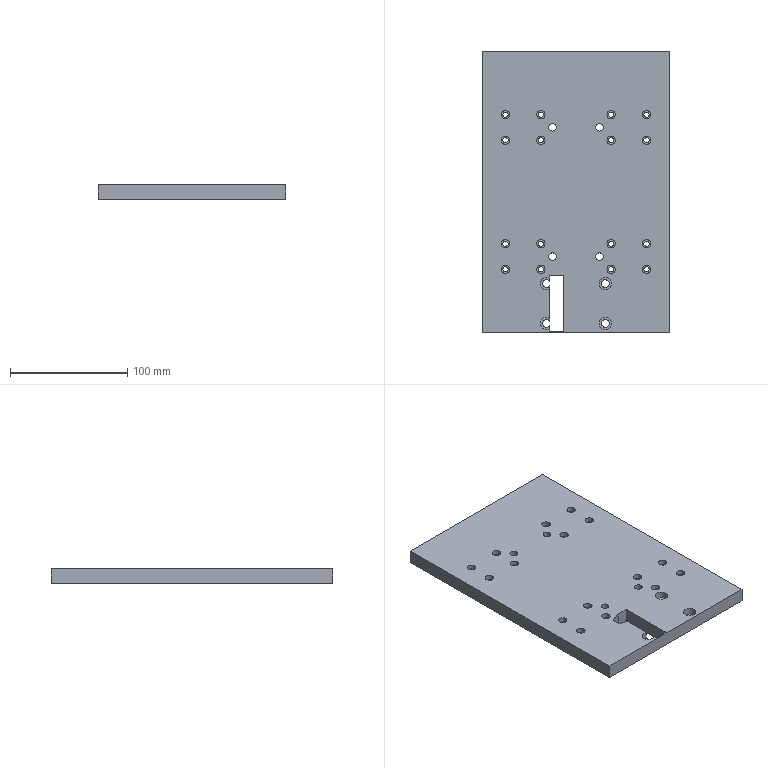Part | SolidWorks | features BaseBody 1 | 1 solid | 116 faces | box 160 x 240 x 12 mm | volume 444930 mm3 | cylinder 84 | plane 32 | commonest cylinder face diameters 4.5 x32 7.2 x32 6.5 x14 10.6 x6